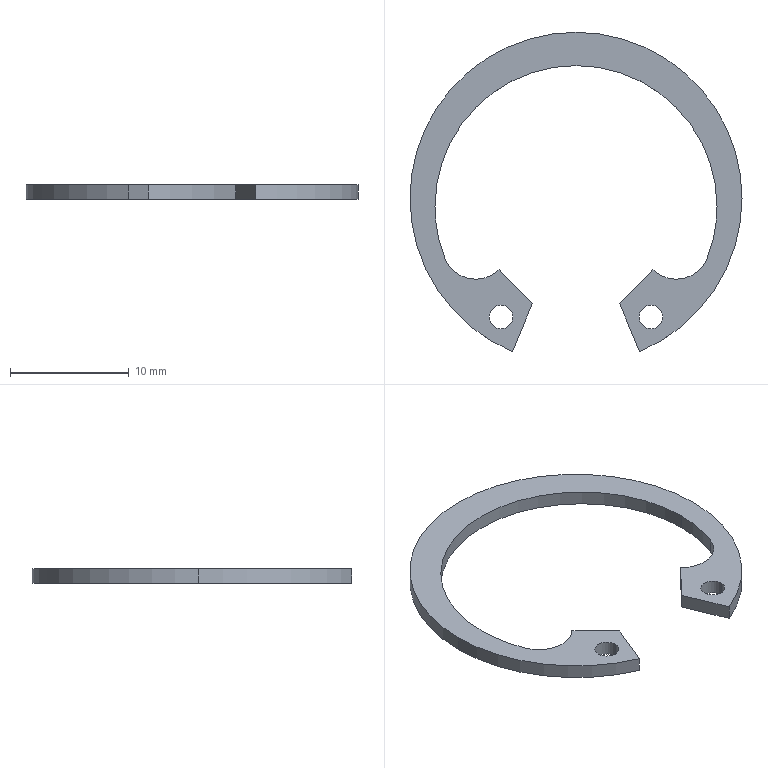Part | SolidWorks | features Extrusion 1 | 1 solid | 18 faces | box 27.9 x 26.838 x 1.2 mm | volume 223.343 mm3 | cylinder 12 | plane 6 | commonest cylinder face diameters 2 x4 23.7 x3 27.9 x3 5.6 x2
STEP:
#1=CARTESIAN_POINT('',(5.298,-9.979,1.2));
#2=VERTEX_POINT('',#1);
#3=CARTESIAN_POINT('',(7.298,-9.979,1.2));
#4=VERTEX_POINT('',#3);
#5=CARTESIAN_POINT('',(6.298,-9.979,1.2));
#6=DIRECTION('',(0.,0.,1.));
#7=DIRECTION('',(-1.,0.,0.));
#8=AXIS2_PLACEMENT_3D('',#5,#6,#7);
#9=CIRCLE('',#8,1.);
#10=EDGE_CURVE('',#2,#4,#9,.T.);
#11=ORIENTED_EDGE('',*,*,#10,.T.);
#12=CARTESIAN_POINT('',(7.298,-9.979,0.));
#13=VERTEX_POINT('',#12);
#14=CARTESIAN_POINT('',(7.298,-9.979,1.2));
#15=DIRECTION('',(0.,0.,-1.));
#16=VECTOR('',#15,1000.);
#17=LINE('',#14,#16);
#18=EDGE_CURVE('',#4,#13,#17,.T.);
#19=ORIENTED_EDGE('',*,*,#18,.T.);
#20=CARTESIAN_POINT('',(5.298,-9.979,0.));
#21=VERTEX_POINT('',#20);
#22=CARTESIAN_POINT('',(6.298,-9.979,0.));
#23=DIRECTION('',(0.,0.,1.));
#24=DIRECTION('',(-1.,0.,0.));
#25=AXIS2_PLACEMENT_3D('',#22,#23,#24);
#26=CIRCLE('',#25,1.);
#27=EDGE_CURVE('',#21,#13,#26,.T.);
#28=ORIENTED_EDGE('',*,*,#27,.F.);
#29=CARTESIAN_POINT('',(5.298,-9.979,1.2));
#30=DIRECTION('',(0.,0.,-1.));
#31=VECTOR('',#30,1000.);
#32=LINE('',#29,#31);
#33=EDGE_CURVE('',#2,#21,#32,.T.);
#34=ORIENTED_EDGE('',*,*,#33,.F.);
#35=EDGE_LOOP('',(#11,#19,#28,#34));
#36=FACE_OUTER_BOUND('',#35,.T.);
#37=CARTESIAN_POINT('',(6.298,-9.979,1.2));
#38=DIRECTION('',(0.,0.,-1.));
#39=DIRECTION('',(-1.,0.,0.));
#40=AXIS2_PLACEMENT_3D('',#37,#38,#39);
#41=CYLINDRICAL_SURFACE('',#40,1.);
#42=ADVANCED_FACE('',(#36),#41,.F.);
#43=CARTESIAN_POINT('',(-7.298,-9.979,1.2));
#44=VERTEX_POINT('',#43);
#45=CARTESIAN_POINT('',(-5.298,-9.979,1.2));
#46=VERTEX_POINT('',#45);
#47=CARTESIAN_POINT('',(-6.298,-9.979,1.2));
#48=DIRECTION('',(0.,0.,1.));
#49=DIRECTION('',(1.,0.,0.));
#50=AXIS2_PLACEMENT_3D('',#47,#48,#49);
#51=CIRCLE('',#50,1.);
#52=EDGE_CURVE('',#44,#46,#51,.T.);
#53=ORIENTED_EDGE('',*,*,#52,.T.);
#54=CARTESIAN_POINT('',(-5.298,-9.979,0.));
#55=VERTEX_POINT('',#54);
#56=CARTESIAN_POINT('',(-5.298,-9.979,1.2));
#57=DIRECTION('',(0.,0.,-1.));
#58=VECTOR('',#57,1000.);
#59=LINE('',#56,#58);
#60=EDGE_CURVE('',#46,#55,#59,.T.);
#61=ORIENTED_EDGE('',*,*,#60,.T.);
#62=CARTESIAN_POINT('',(-7.298,-9.979,0.));
#63=VERTEX_POINT('',#62);
#64=CARTESIAN_POINT('',(-6.298,-9.979,0.));
#65=DIRECTION('',(0.,0.,1.));
#66=DIRECTION('',(1.,0.,0.));
#67=AXIS2_PLACEMENT_3D('',#64,#65,#66);
#68=CIRCLE('',#67,1.);
#69=EDGE_CURVE('',#63,#55,#68,.T.);
#70=ORIENTED_EDGE('',*,*,#69,.F.);
#71=CARTESIAN_POINT('',(-7.298,-9.979,1.2));
#72=DIRECTION('',(0.,0.,-1.));
#73=VECTOR('',#72,1000.);
#74=LINE('',#71,#73);
#75=EDGE_CURVE('',#44,#63,#74,.T.);
#76=ORIENTED_EDGE('',*,*,#75,.F.);
#77=EDGE_LOOP('',(#53,#61,#70,#76));
#78=FACE_OUTER_BOUND('',#77,.T.);
#79=CARTESIAN_POINT('',(-6.298,-9.979,1.2));
#80=DIRECTION('',(0.,0.,-1.));
#81=DIRECTION('',(-1.,0.,0.));
#82=AXIS2_PLACEMENT_3D('',#79,#80,#81);
#83=CYLINDRICAL_SURFACE('',#82,1.);
#84=ADVANCED_FACE('',(#78),#83,.F.);
#85=CARTESIAN_POINT('',(11.85,-0.7,1.2));
#86=VERTEX_POINT('',#85);
#87=CARTESIAN_POINT('',(11.034,-5.022,1.2));
#88=VERTEX_POINT('',#87);
#89=CARTESIAN_POINT('',(0.,-0.7,1.2));
#90=DIRECTION('',(0.,0.,-1.));
#91=DIRECTION('',(1.,0.,0.));
#92=AXIS2_PLACEMENT_3D('',#89,#90,#91);
#93=CIRCLE('',#92,11.85);
#94=EDGE_CURVE('',#86,#88,#93,.T.);
#95=ORIENTED_EDGE('',*,*,#94,.F.);
#96=CARTESIAN_POINT('',(11.85,-0.7,0.));
#97=VERTEX_POINT('',#96);
#98=CARTESIAN_POINT('',(11.85,-0.7,1.2));
#99=DIRECTION('',(0.,0.,-1.));
#100=VECTOR('',#99,1000.);
#101=LINE('',#98,#100);
#102=EDGE_CURVE('',#86,#97,#101,.T.);
#103=ORIENTED_EDGE('',*,*,#102,.T.);
#104=CARTESIAN_POINT('',(11.034,-5.022,0.));
#105=VERTEX_POINT('',#104);
#106=CARTESIAN_POINT('',(0.,-0.7,0.));
#107=DIRECTION('',(0.,0.,-1.));
#108=DIRECTION('',(1.,0.,0.));
#109=AXIS2_PLACEMENT_3D('',#106,#107,#108);
#110=CIRCLE('',#109,11.85);
#111=EDGE_CURVE('',#97,#105,#110,.T.);
#112=ORIENTED_EDGE('',*,*,#111,.T.);
#113=CARTESIAN_POINT('',(11.034,-5.022,1.2));
#114=DIRECTION('',(0.,0.,-1.));
#115=VECTOR('',#114,1000.);
#116=LINE('',#113,#115);
#117=EDGE_CURVE('',#88,#105,#116,.T.);
#118=ORIENTED_EDGE('',*,*,#117,.F.);
#119=EDGE_LOOP('',(#95,#103,#112,#118));
#120=FACE_OUTER_BOUND('',#119,.T.);
#121=CARTESIAN_POINT('',(0.,-0.7,1.2));
#122=DIRECTION('',(0.,0.,-1.));
#123=DIRECTION('',(-1.,0.,0.));
#124=AXIS2_PLACEMENT_3D('',#121,#122,#123);
#125=CYLINDRICAL_SURFACE('',#124,11.85);
#126=ADVANCED_FACE('',(#120),#125,.F.);
#127=ORIENTED_EDGE('',*,*,#102,.F.);
#128=CARTESIAN_POINT('',(-11.85,-0.7,1.2));
#129=VERTEX_POINT('',#128);
#130=CARTESIAN_POINT('',(0.,-0.7,1.2));
#131=DIRECTION('',(0.,0.,-1.));
#132=DIRECTION('',(1.,0.,0.));
#133=AXIS2_PLACEMENT_3D('',#130,#131,#132);
#134=CIRCLE('',#133,11.85);
#135=EDGE_CURVE('',#129,#86,#134,.T.);
#136=ORIENTED_EDGE('',*,*,#135,.F.);
#137=CARTESIAN_POINT('',(-11.85,-0.7,0.));
#138=VERTEX_POINT('',#137);
#139=CARTESIAN_POINT('',(-11.85,-0.7,1.2));
#140=DIRECTION('',(0.,0.,-1.));
#141=VECTOR('',#140,1000.);
#142=LINE('',#139,#141);
#143=EDGE_CURVE('',#129,#138,#142,.T.);
#144=ORIENTED_EDGE('',*,*,#143,.T.);
#145=CARTESIAN_POINT('',(0.,-0.7,0.));
#146=DIRECTION('',(0.,0.,-1.));
#147=DIRECTION('',(1.,0.,0.));
#148=AXIS2_PLACEMENT_3D('',#145,#146,#147);
#149=CIRCLE('',#148,11.85);
#150=EDGE_CURVE('',#138,#97,#149,.T.);
#151=ORIENTED_EDGE('',*,*,#150,.T.);
#152=EDGE_LOOP('',(#127,#136,#144,#151));
#153=FACE_OUTER_BOUND('',#152,.T.);
#154=CARTESIAN_POINT('',(0.,-0.7,1.2));
#155=DIRECTION('',(0.,0.,-1.));
#156=DIRECTION('',(-1.,0.,0.));
#157=AXIS2_PLACEMENT_3D('',#154,#155,#156);
#158=CYLINDRICAL_SURFACE('',#157,11.85);
#159=ADVANCED_FACE('',(#153),#158,.F.);
#160=CARTESIAN_POINT('',(13.95,0.,1.2));
#161=VERTEX_POINT('',#160);
#162=CARTESIAN_POINT('',(-13.95,0.,1.2));
#163=VERTEX_POINT('',#162);
#164=CARTESIAN_POINT('',(0.,0.,1.2));
#165=DIRECTION('',(0.,0.,1.));
#166=DIRECTION('',(1.,0.,0.));
#167=AXIS2_PLACEMENT_3D('',#164,#165,#166);
#168=CIRCLE('',#167,13.95);
#169=EDGE_CURVE('',#161,#163,#168,.T.);
#170=ORIENTED_EDGE('',*,*,#169,.F.);
#171=CARTESIAN_POINT('',(13.95,0.,0.));
#172=VERTEX_POINT('',#171);
#173=CARTESIAN_POINT('',(13.95,0.,1.2));
#174=DIRECTION('',(0.,0.,-1.));
#175=VECTOR('',#174,1000.);
#176=LINE('',#173,#175);
#177=EDGE_CURVE('',#161,#172,#176,.T.);
#178=ORIENTED_EDGE('',*,*,#177,.T.);
#179=CARTESIAN_POINT('',(-13.95,0.,0.));
#180=VERTEX_POINT('',#179);
#181=CARTESIAN_POINT('',(0.,0.,0.));
#182=DIRECTION('',(0.,0.,1.));
#183=DIRECTION('',(1.,0.,0.));
#184=AXIS2_PLACEMENT_3D('',#181,#182,#183);
#185=CIRCLE('',#184,13.95);
#186=EDGE_CURVE('',#172,#180,#185,.T.);
#187=ORIENTED_EDGE('',*,*,#186,.T.);
#188=CARTESIAN_POINT('',(-13.95,0.,1.2));
#189=DIRECTION('',(0.,0.,-1.));
#190=VECTOR('',#189,1000.);
#191=LINE('',#188,#190);
#192=EDGE_CURVE('',#163,#180,#191,.T.);
#193=ORIENTED_EDGE('',*,*,#192,.F.);
#194=EDGE_LOOP('',(#170,#178,#187,#193));
#195=FACE_OUTER_BOUND('',#194,.T.);
#196=CARTESIAN_POINT('',(0.,0.,1.2));
#197=DIRECTION('',(0.,0.,-1.));
#198=DIRECTION('',(-1.,0.,0.));
#199=AXIS2_PLACEMENT_3D('',#196,#197,#198);
#200=CYLINDRICAL_SURFACE('',#199,13.95);
#201=ADVANCED_FACE('',(#195),#200,.T.);
#202=CARTESIAN_POINT('',(-5.338,-12.888,1.2));
#203=VERTEX_POINT('',#202);
#204=CARTESIAN_POINT('',(0.,0.,1.2));
#205=DIRECTION('',(0.,0.,1.));
#206=DIRECTION('',(1.,0.,0.));
#207=AXIS2_PLACEMENT_3D('',#204,#205,#206);
#208=CIRCLE('',#207,13.95);
#209=EDGE_CURVE('',#163,#203,#208,.T.);
#210=ORIENTED_EDGE('',*,*,#209,.F.);
#211=ORIENTED_EDGE('',*,*,#192,.T.);
#212=CARTESIAN_POINT('',(-5.338,-12.888,0.));
#213=VERTEX_POINT('',#212);
#214=CARTESIAN_POINT('',(0.,0.,0.));
#215=DIRECTION('',(0.,0.,1.));
#216=DIRECTION('',(1.,0.,0.));
#217=AXIS2_PLACEMENT_3D('',#214,#215,#216);
#218=CIRCLE('',#217,13.95);
#219=EDGE_CURVE('',#180,#213,#218,.T.);
#220=ORIENTED_EDGE('',*,*,#219,.T.);
#221=CARTESIAN_POINT('',(-5.338,-12.888,1.2));
#222=DIRECTION('',(0.,0.,-1.));
#223=VECTOR('',#222,1000.);
#224=LINE('',#221,#223);
#225=EDGE_CURVE('',#203,#213,#224,.T.);
#226=ORIENTED_EDGE('',*,*,#225,.F.);
#227=EDGE_LOOP('',(#210,#211,#220,#226));
#228=FACE_OUTER_BOUND('',#227,.T.);
#229=CARTESIAN_POINT('',(0.,0.,1.2));
#230=DIRECTION('',(0.,0.,-1.));
#231=DIRECTION('',(-1.,0.,0.));
#232=AXIS2_PLACEMENT_3D('',#229,#230,#231);
#233=CYLINDRICAL_SURFACE('',#232,13.95);
#234=ADVANCED_FACE('',(#228),#233,.T.);
#235=ORIENTED_EDGE('',*,*,#52,.F.);
#236=CARTESIAN_POINT('',(-6.298,-9.979,1.2));
#237=DIRECTION('',(0.,0.,1.));
#238=DIRECTION('',(1.,0.,0.));
#239=AXIS2_PLACEMENT_3D('',#236,#237,#238);
#240=CIRCLE('',#239,1.);
#241=EDGE_CURVE('',#46,#44,#240,.T.);
#242=ORIENTED_EDGE('',*,*,#241,.F.);
#243=EDGE_LOOP('',(#235,#242));
#244=FACE_BOUND('',#243,.T.);
#245=CARTESIAN_POINT('',(5.338,-12.888,1.2));
#246=VERTEX_POINT('',#245);
#247=CARTESIAN_POINT('',(0.,0.,1.2));
#248=DIRECTION('',(0.,0.,1.));
#249=DIRECTION('',(1.,0.,0.));
#250=AXIS2_PLACEMENT_3D('',#247,#248,#249);
#251=CIRCLE('',#250,13.95);
#252=EDGE_CURVE('',#246,#161,#251,.T.);
#253=ORIENTED_EDGE('',*,*,#252,.T.);
#254=ORIENTED_EDGE('',*,*,#169,.T.);
#255=ORIENTED_EDGE('',*,*,#209,.T.);
#256=CARTESIAN_POINT('',(-3.67,-8.86,1.2));
#257=VERTEX_POINT('',#256);
#258=CARTESIAN_POINT('',(-3.67,-8.86,1.2));
#259=DIRECTION('',(0.3827,0.9239,0.));
#260=VECTOR('',#259,1000.);
#261=LINE('',#258,#260);
#262=EDGE_CURVE('',#203,#257,#261,.T.);
#263=ORIENTED_EDGE('',*,*,#262,.T.);
#264=CARTESIAN_POINT('',(-6.468,-6.002,1.2));
#265=VERTEX_POINT('',#264);
#266=CARTESIAN_POINT('',(-6.468,-6.002,1.2));
#267=DIRECTION('',(-0.6995,0.7146,0.));
#268=VECTOR('',#267,1000.);
#269=LINE('',#266,#268);
#270=EDGE_CURVE('',#257,#265,#269,.T.);
#271=ORIENTED_EDGE('',*,*,#270,.T.);
#272=CARTESIAN_POINT('',(-11.034,-5.022,1.2));
#273=VERTEX_POINT('',#272);
#274=CARTESIAN_POINT('',(-8.427,-4.001,1.2));
#275=DIRECTION('',(0.,0.,-1.));
#276=DIRECTION('',(1.,0.,0.));
#277=AXIS2_PLACEMENT_3D('',#274,#275,#276);
#278=CIRCLE('',#277,2.8);
#279=EDGE_CURVE('',#265,#273,#278,.T.);
#280=ORIENTED_EDGE('',*,*,#279,.T.);
#281=CARTESIAN_POINT('',(0.,-0.7,1.2));
#282=DIRECTION('',(0.,0.,-1.));
#283=DIRECTION('',(1.,0.,0.));
#284=AXIS2_PLACEMENT_3D('',#281,#282,#283);
#285=CIRCLE('',#284,11.85);
#286=EDGE_CURVE('',#273,#129,#285,.T.);
#287=ORIENTED_EDGE('',*,*,#286,.T.);
#288=ORIENTED_EDGE('',*,*,#135,.T.);
#289=ORIENTED_EDGE('',*,*,#94,.T.);
#290=CARTESIAN_POINT('',(6.468,-6.002,1.2));
#291=VERTEX_POINT('',#290);
#292=CARTESIAN_POINT('',(8.427,-4.001,1.2));
#293=DIRECTION('',(0.,0.,-1.));
#294=DIRECTION('',(-1.,0.,0.));
#295=AXIS2_PLACEMENT_3D('',#292,#293,#294);
#296=CIRCLE('',#295,2.8);
#297=EDGE_CURVE('',#88,#291,#296,.T.);
#298=ORIENTED_EDGE('',*,*,#297,.T.);
#299=CARTESIAN_POINT('',(3.67,-8.86,1.2));
#300=VERTEX_POINT('',#299);
#301=CARTESIAN_POINT('',(6.468,-6.002,1.2));
#302=DIRECTION('',(-0.6995,-0.7146,0.));
#303=VECTOR('',#302,1000.);
#304=LINE('',#301,#303);
#305=EDGE_CURVE('',#291,#300,#304,.T.);
#306=ORIENTED_EDGE('',*,*,#305,.T.);
#307=CARTESIAN_POINT('',(3.67,-8.86,1.2));
#308=DIRECTION('',(0.3827,-0.9239,0.));
#309=VECTOR('',#308,1000.);
#310=LINE('',#307,#309);
#311=EDGE_CURVE('',#300,#246,#310,.T.);
#312=ORIENTED_EDGE('',*,*,#311,.T.);
#313=EDGE_LOOP('',(#253,#254,#255,#263,#271,#280,#287,#288,#289,#298,#306,#312));
#314=FACE_OUTER_BOUND('',#313,.T.);
#315=ORIENTED_EDGE('',*,*,#10,.F.);
#316=CARTESIAN_POINT('',(6.298,-9.979,1.2));
#317=DIRECTION('',(0.,0.,1.));
#318=DIRECTION('',(-1.,0.,0.));
#319=AXIS2_PLACEMENT_3D('',#316,#317,#318);
#320=CIRCLE('',#319,1.);
#321=EDGE_CURVE('',#4,#2,#320,.T.);
#322=ORIENTED_EDGE('',*,*,#321,.F.);
#323=EDGE_LOOP('',(#315,#322));
#324=FACE_BOUND('',#323,.T.);
#325=CARTESIAN_POINT('',(0.,0.,1.2));
#326=DIRECTION('',(0.,0.,1.));
#327=DIRECTION('',(1.,0.,0.));
#328=AXIS2_PLACEMENT_3D('',#325,#326,#327);
#329=PLANE('',#328);
#330=ADVANCED_FACE('',(#244,#314,#324),#329,.T.);
#331=CARTESIAN_POINT('',(5.338,-12.888,0.));
#332=VERTEX_POINT('',#331);
#333=CARTESIAN_POINT('',(0.,0.,0.));
#334=DIRECTION('',(0.,0.,1.));
#335=DIRECTION('',(1.,0.,0.));
#336=AXIS2_PLACEMENT_3D('',#333,#334,#335);
#337=CIRCLE('',#336,13.95);
#338=EDGE_CURVE('',#332,#172,#337,.T.);
#339=ORIENTED_EDGE('',*,*,#338,.F.);
#340=CARTESIAN_POINT('',(3.67,-8.86,0.));
#341=VERTEX_POINT('',#340);
#342=CARTESIAN_POINT('',(3.67,-8.86,0.));
#343=DIRECTION('',(0.3827,-0.9239,0.));
#344=VECTOR('',#343,1000.);
#345=LINE('',#342,#344);
#346=EDGE_CURVE('',#341,#332,#345,.T.);
#347=ORIENTED_EDGE('',*,*,#346,.F.);
#348=CARTESIAN_POINT('',(6.468,-6.002,0.));
#349=VERTEX_POINT('',#348);
#350=CARTESIAN_POINT('',(6.468,-6.002,0.));
#351=DIRECTION('',(-0.6995,-0.7146,0.));
#352=VECTOR('',#351,1000.);
#353=LINE('',#350,#352);
#354=EDGE_CURVE('',#349,#341,#353,.T.);
#355=ORIENTED_EDGE('',*,*,#354,.F.);
#356=CARTESIAN_POINT('',(8.427,-4.001,0.));
#357=DIRECTION('',(0.,0.,-1.));
#358=DIRECTION('',(-1.,0.,0.));
#359=AXIS2_PLACEMENT_3D('',#356,#357,#358);
#360=CIRCLE('',#359,2.8);
#361=EDGE_CURVE('',#105,#349,#360,.T.);
#362=ORIENTED_EDGE('',*,*,#361,.F.);
#363=ORIENTED_EDGE('',*,*,#111,.F.);
#364=ORIENTED_EDGE('',*,*,#150,.F.);
#365=CARTESIAN_POINT('',(-11.034,-5.022,0.));
#366=VERTEX_POINT('',#365);
#367=CARTESIAN_POINT('',(0.,-0.7,0.));
#368=DIRECTION('',(0.,0.,-1.));
#369=DIRECTION('',(1.,0.,0.));
#370=AXIS2_PLACEMENT_3D('',#367,#368,#369);
#371=CIRCLE('',#370,11.85);
#372=EDGE_CURVE('',#366,#138,#371,.T.);
#373=ORIENTED_EDGE('',*,*,#372,.F.);
#374=CARTESIAN_POINT('',(-6.468,-6.002,0.));
#375=VERTEX_POINT('',#374);
#376=CARTESIAN_POINT('',(-8.427,-4.001,0.));
#377=DIRECTION('',(0.,0.,-1.));
#378=DIRECTION('',(1.,0.,0.));
#379=AXIS2_PLACEMENT_3D('',#376,#377,#378);
#380=CIRCLE('',#379,2.8);
#381=EDGE_CURVE('',#375,#366,#380,.T.);
#382=ORIENTED_EDGE('',*,*,#381,.F.);
#383=CARTESIAN_POINT('',(-3.67,-8.86,0.));
#384=VERTEX_POINT('',#383);
#385=CARTESIAN_POINT('',(-6.468,-6.002,0.));
#386=DIRECTION('',(-0.6995,0.7146,0.));
#387=VECTOR('',#386,1000.);
#388=LINE('',#385,#387);
#389=EDGE_CURVE('',#384,#375,#388,.T.);
#390=ORIENTED_EDGE('',*,*,#389,.F.);
#391=CARTESIAN_POINT('',(-3.67,-8.86,0.));
#392=DIRECTION('',(0.3827,0.9239,0.));
#393=VECTOR('',#392,1000.);
#394=LINE('',#391,#393);
#395=EDGE_CURVE('',#213,#384,#394,.T.);
#396=ORIENTED_EDGE('',*,*,#395,.F.);
#397=ORIENTED_EDGE('',*,*,#219,.F.);
#398=ORIENTED_EDGE('',*,*,#186,.F.);
#399=EDGE_LOOP('',(#339,#347,#355,#362,#363,#364,#373,#382,#390,#396,#397,#398));
#400=FACE_OUTER_BOUND('',#399,.T.);
#401=ORIENTED_EDGE('',*,*,#69,.T.);
#402=CARTESIAN_POINT('',(-6.298,-9.979,0.));
#403=DIRECTION('',(0.,0.,1.));
#404=DIRECTION('',(1.,0.,0.));
#405=AXIS2_PLACEMENT_3D('',#402,#403,#404);
#406=CIRCLE('',#405,1.);
#407=EDGE_CURVE('',#55,#63,#406,.T.);
#408=ORIENTED_EDGE('',*,*,#407,.T.);
#409=EDGE_LOOP('',(#401,#408));
#410=FACE_BOUND('',#409,.T.);
#411=ORIENTED_EDGE('',*,*,#27,.T.);
#412=CARTESIAN_POINT('',(6.298,-9.979,0.));
#413=DIRECTION('',(0.,0.,1.));
#414=DIRECTION('',(-1.,0.,0.));
#415=AXIS2_PLACEMENT_3D('',#412,#413,#414);
#416=CIRCLE('',#415,1.);
#417=EDGE_CURVE('',#13,#21,#416,.T.);
#418=ORIENTED_EDGE('',*,*,#417,.T.);
#419=EDGE_LOOP('',(#411,#418));
#420=FACE_BOUND('',#419,.T.);
#421=CARTESIAN_POINT('',(0.,0.,0.));
#422=DIRECTION('',(0.,0.,1.));
#423=DIRECTION('',(1.,0.,0.));
#424=AXIS2_PLACEMENT_3D('',#421,#422,#423);
#425=PLANE('',#424);
#426=ADVANCED_FACE('',(#400,#410,#420),#425,.F.);
#427=ORIENTED_EDGE('',*,*,#177,.F.);
#428=ORIENTED_EDGE('',*,*,#252,.F.);
#429=CARTESIAN_POINT('',(5.338,-12.888,1.2));
#430=DIRECTION('',(0.,0.,-1.));
#431=VECTOR('',#430,1000.);
#432=LINE('',#429,#431);
#433=EDGE_CURVE('',#246,#332,#432,.T.);
#434=ORIENTED_EDGE('',*,*,#433,.T.);
#435=ORIENTED_EDGE('',*,*,#338,.T.);
#436=EDGE_LOOP('',(#427,#428,#434,#435));
#437=FACE_OUTER_BOUND('',#436,.T.);
#438=CARTESIAN_POINT('',(0.,0.,1.2));
#439=DIRECTION('',(0.,0.,-1.));
#440=DIRECTION('',(-1.,0.,0.));
#441=AXIS2_PLACEMENT_3D('',#438,#439,#440);
#442=CYLINDRICAL_SURFACE('',#441,13.95);
#443=ADVANCED_FACE('',(#437),#442,.T.);
#444=ORIENTED_EDGE('',*,*,#395,.T.);
#445=CARTESIAN_POINT('',(-3.67,-8.86,1.2));
#446=DIRECTION('',(0.,0.,-1.));
#447=VECTOR('',#446,1000.);
#448=LINE('',#445,#447);
#449=EDGE_CURVE('',#257,#384,#448,.T.);
#450=ORIENTED_EDGE('',*,*,#449,.F.);
#451=ORIENTED_EDGE('',*,*,#262,.F.);
#452=ORIENTED_EDGE('',*,*,#225,.T.);
#453=EDGE_LOOP('',(#444,#450,#451,#452));
#454=FACE_OUTER_BOUND('',#453,.T.);
#455=CARTESIAN_POINT('',(-3.67,-8.86,1.2));
#456=DIRECTION('',(-0.9239,0.3827,0.));
#457=DIRECTION('',(-0.3827,-0.9239,0.));
#458=AXIS2_PLACEMENT_3D('',#455,#456,#457);
#459=PLANE('',#458);
#460=ADVANCED_FACE('',(#454),#459,.F.);
#461=ORIENTED_EDGE('',*,*,#389,.T.);
#462=CARTESIAN_POINT('',(-6.468,-6.002,1.2));
#463=DIRECTION('',(0.,0.,-1.));
#464=VECTOR('',#463,1000.);
#465=LINE('',#462,#464);
#466=EDGE_CURVE('',#265,#375,#465,.T.);
#467=ORIENTED_EDGE('',*,*,#466,.F.);
#468=ORIENTED_EDGE('',*,*,#270,.F.);
#469=ORIENTED_EDGE('',*,*,#449,.T.);
#470=EDGE_LOOP('',(#461,#467,#468,#469));
#471=FACE_OUTER_BOUND('',#470,.T.);
#472=CARTESIAN_POINT('',(-6.468,-6.002,1.2));
#473=DIRECTION('',(-0.7146,-0.6995,0.));
#474=DIRECTION('',(0.6995,-0.7146,0.));
#475=AXIS2_PLACEMENT_3D('',#472,#473,#474);
#476=PLANE('',#475);
#477=ADVANCED_FACE('',(#471),#476,.F.);
#478=ORIENTED_EDGE('',*,*,#381,.T.);
#479=CARTESIAN_POINT('',(-11.034,-5.022,1.2));
#480=DIRECTION('',(0.,0.,-1.));
#481=VECTOR('',#480,1000.);
#482=LINE('',#479,#481);
#483=EDGE_CURVE('',#273,#366,#482,.T.);
#484=ORIENTED_EDGE('',*,*,#483,.F.);
#485=ORIENTED_EDGE('',*,*,#279,.F.);
#486=ORIENTED_EDGE('',*,*,#466,.T.);
#487=EDGE_LOOP('',(#478,#484,#485,#486));
#488=FACE_OUTER_BOUND('',#487,.T.);
#489=CARTESIAN_POINT('',(-8.427,-4.001,1.2));
#490=DIRECTION('',(0.,0.,-1.));
#491=DIRECTION('',(-1.,0.,0.));
#492=AXIS2_PLACEMENT_3D('',#489,#490,#491);
#493=CYLINDRICAL_SURFACE('',#492,2.8);
#494=ADVANCED_FACE('',(#488),#493,.F.);
#495=ORIENTED_EDGE('',*,*,#143,.F.);
#496=ORIENTED_EDGE('',*,*,#286,.F.);
#497=ORIENTED_EDGE('',*,*,#483,.T.);
#498=ORIENTED_EDGE('',*,*,#372,.T.);
#499=EDGE_LOOP('',(#495,#496,#497,#498));
#500=FACE_OUTER_BOUND('',#499,.T.);
#501=CARTESIAN_POINT('',(0.,-0.7,1.2));
#502=DIRECTION('',(0.,0.,-1.));
#503=DIRECTION('',(-1.,0.,0.));
#504=AXIS2_PLACEMENT_3D('',#501,#502,#503);
#505=CYLINDRICAL_SURFACE('',#504,11.85);
#506=ADVANCED_FACE('',(#500),#505,.F.);
#507=ORIENTED_EDGE('',*,*,#361,.T.);
#508=CARTESIAN_POINT('',(6.468,-6.002,1.2));
#509=DIRECTION('',(0.,0.,-1.));
#510=VECTOR('',#509,1000.);
#511=LINE('',#508,#510);
#512=EDGE_CURVE('',#291,#349,#511,.T.);
#513=ORIENTED_EDGE('',*,*,#512,.F.);
#514=ORIENTED_EDGE('',*,*,#297,.F.);
#515=ORIENTED_EDGE('',*,*,#117,.T.);
#516=EDGE_LOOP('',(#507,#513,#514,#515));
#517=FACE_OUTER_BOUND('',#516,.T.);
#518=CARTESIAN_POINT('',(8.427,-4.001,1.2));
#519=DIRECTION('',(0.,0.,-1.));
#520=DIRECTION('',(-1.,0.,0.));
#521=AXIS2_PLACEMENT_3D('',#518,#519,#520);
#522=CYLINDRICAL_SURFACE('',#521,2.8);
#523=ADVANCED_FACE('',(#517),#522,.F.);
#524=ORIENTED_EDGE('',*,*,#354,.T.);
#525=CARTESIAN_POINT('',(3.67,-8.86,1.2));
#526=DIRECTION('',(0.,0.,-1.));
#527=VECTOR('',#526,1000.);
#528=LINE('',#525,#527);
#529=EDGE_CURVE('',#300,#341,#528,.T.);
#530=ORIENTED_EDGE('',*,*,#529,.F.);
#531=ORIENTED_EDGE('',*,*,#305,.F.);
#532=ORIENTED_EDGE('',*,*,#512,.T.);
#533=EDGE_LOOP('',(#524,#530,#531,#532));
#534=FACE_OUTER_BOUND('',#533,.T.);
#535=CARTESIAN_POINT('',(6.468,-6.002,1.2));
#536=DIRECTION('',(0.7146,-0.6995,0.));
#537=DIRECTION('',(0.6995,0.7146,0.));
#538=AXIS2_PLACEMENT_3D('',#535,#536,#537);
#539=PLANE('',#538);
#540=ADVANCED_FACE('',(#534),#539,.F.);
#541=ORIENTED_EDGE('',*,*,#346,.T.);
#542=ORIENTED_EDGE('',*,*,#433,.F.);
#543=ORIENTED_EDGE('',*,*,#311,.F.);
#544=ORIENTED_EDGE('',*,*,#529,.T.);
#545=EDGE_LOOP('',(#541,#542,#543,#544));
#546=FACE_OUTER_BOUND('',#545,.T.);
#547=CARTESIAN_POINT('',(3.67,-8.86,1.2));
#548=DIRECTION('',(0.9239,0.3827,0.));
#549=DIRECTION('',(-0.3827,0.9239,0.));
#550=AXIS2_PLACEMENT_3D('',#547,#548,#549);
#551=PLANE('',#550);
#552=ADVANCED_FACE('',(#546),#551,.F.);
#553=ORIENTED_EDGE('',*,*,#60,.F.);
#554=ORIENTED_EDGE('',*,*,#241,.T.);
#555=ORIENTED_EDGE('',*,*,#75,.T.);
#556=ORIENTED_EDGE('',*,*,#407,.F.);
#557=EDGE_LOOP('',(#553,#554,#555,#556));
#558=FACE_OUTER_BOUND('',#557,.T.);
#559=CARTESIAN_POINT('',(-6.298,-9.979,1.2));
#560=DIRECTION('',(0.,0.,-1.));
#561=DIRECTION('',(-1.,0.,0.));
#562=AXIS2_PLACEMENT_3D('',#559,#560,#561);
#563=CYLINDRICAL_SURFACE('',#562,1.);
#564=ADVANCED_FACE('',(#558),#563,.F.);
#565=ORIENTED_EDGE('',*,*,#18,.F.);
#566=ORIENTED_EDGE('',*,*,#321,.T.);
#567=ORIENTED_EDGE('',*,*,#33,.T.);
#568=ORIENTED_EDGE('',*,*,#417,.F.);
#569=EDGE_LOOP('',(#565,#566,#567,#568));
#570=FACE_OUTER_BOUND('',#569,.T.);
#571=CARTESIAN_POINT('',(6.298,-9.979,1.2));
#572=DIRECTION('',(0.,0.,-1.));
#573=DIRECTION('',(-1.,0.,0.));
#574=AXIS2_PLACEMENT_3D('',#571,#572,#573);
#575=CYLINDRICAL_SURFACE('',#574,1.);
#576=ADVANCED_FACE('',(#570),#575,.F.);
#577=CLOSED_SHELL('',(#42,#84,#126,#159,#201,#234,#330,#426,#443,#460,#477,#494,#506,#523,#540,#552,#564,#576));
#578=MANIFOLD_SOLID_BREP('',#577);
#579=CARTESIAN_POINT('',(0.,0.,0.));
#580=DIRECTION('',(0.,0.,1.));
#581=DIRECTION('',(1.,0.,0.));
#582=AXIS2_PLACEMENT_3D('',#579,#580,#581);
#583=(LENGTH_UNIT()NAMED_UNIT(*)SI_UNIT(.MILLI.,.METRE.));
#584=UNCERTAINTY_MEASURE_WITH_UNIT(LENGTH_MEASURE(0.00001),#583,'','');
#585=(NAMED_UNIT(*)PLANE_ANGLE_UNIT()SI_UNIT($,.RADIAN.));
#586=(NAMED_UNIT(*)SI_UNIT($,.STERADIAN.)SOLID_ANGLE_UNIT());
#587=(GEOMETRIC_REPRESENTATION_CONTEXT(3)GLOBAL_UNCERTAINTY_ASSIGNED_CONTEXT((#584))GLOBAL_UNIT_ASSIGNED_CONTEXT((#583,#585,#586))REPRESENTATION_CONTEXT('',''));
#588=ADVANCED_BREP_SHAPE_REPRESENTATION('',(#578,#582),#587);